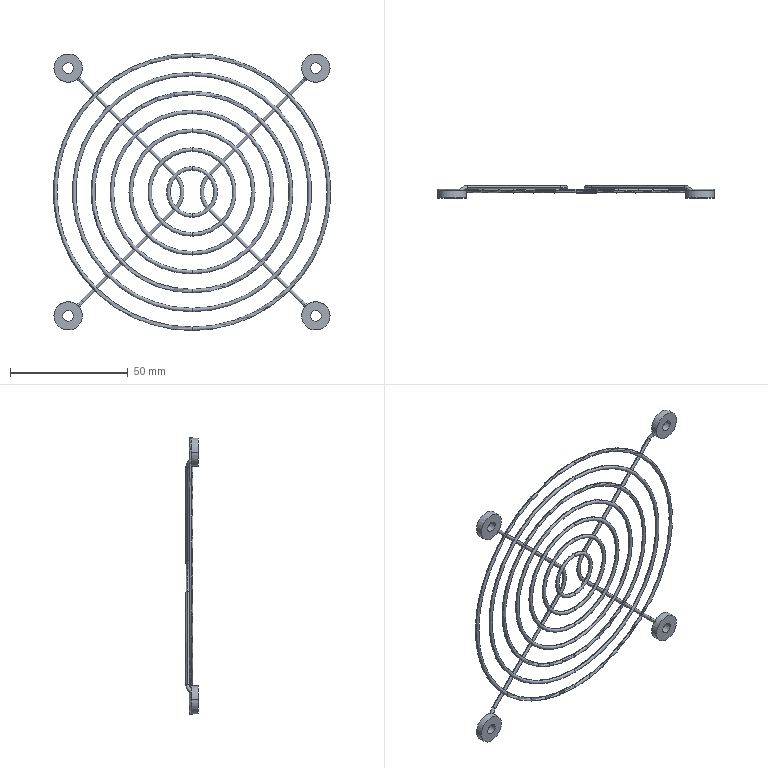Part | SolidWorks | features Boss 1, CompositeCurve 1, MirrorPattern 1, Revolution 1, Sweep 1 | 1 solid | 72 faces | box 117.5 x 5.2 x 117.5 mm | volume 4285 mm3 | torus 40 | cylinder 24 | plane 8 | commonest cylinder face diameters 1.5 x8 4.5 x8 12 x8